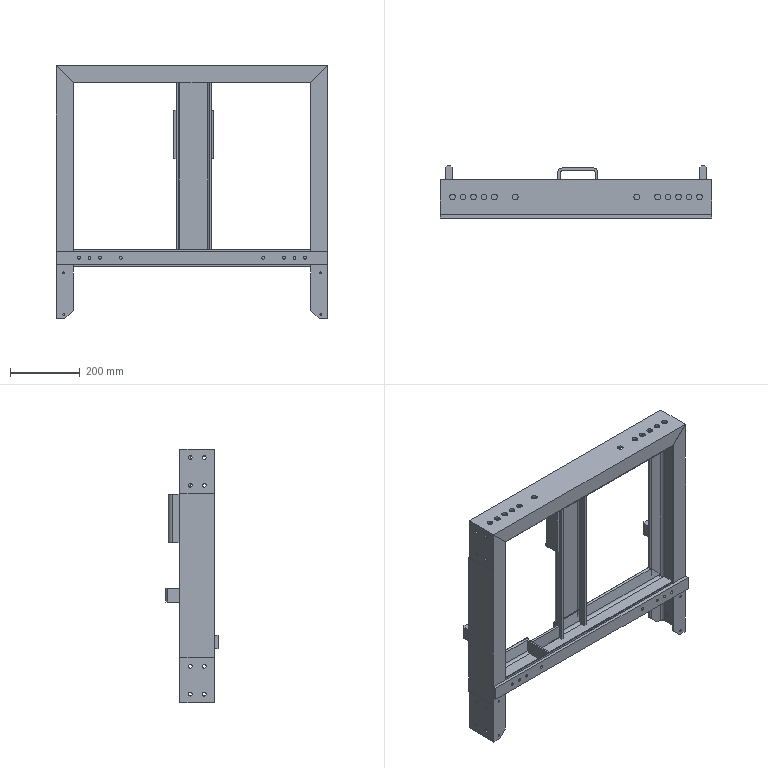Part | SolidWorks | 11 solids | 275 faces | box 782 x 150 x 730 mm | volume 4807451 mm3 | cylinder 141 | plane 134 | commonest cylinder face diameters 8.5 x32 11 x32 16.5 x24 6.8 x16 5 x12 9 x9